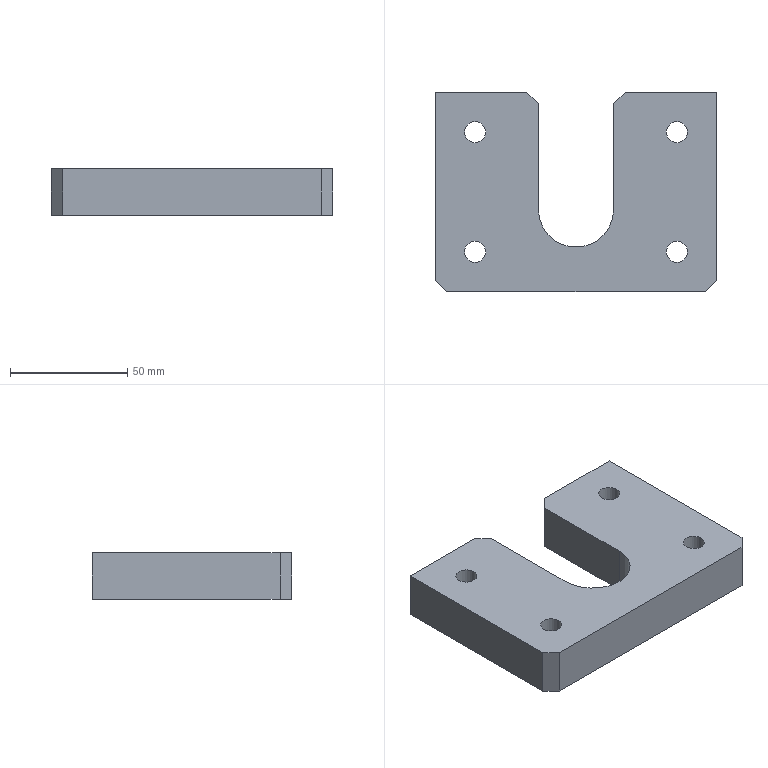Part | STEP file | gslz 2016.10.28-10_id2258_x_t | 1 solid | 26 faces | box 120 x 85 x 20 mm | volume 154255 mm3 | plane 17 | cylinder 9 | commonest cylinder face diameters 9 x4 14 x4 32 x1